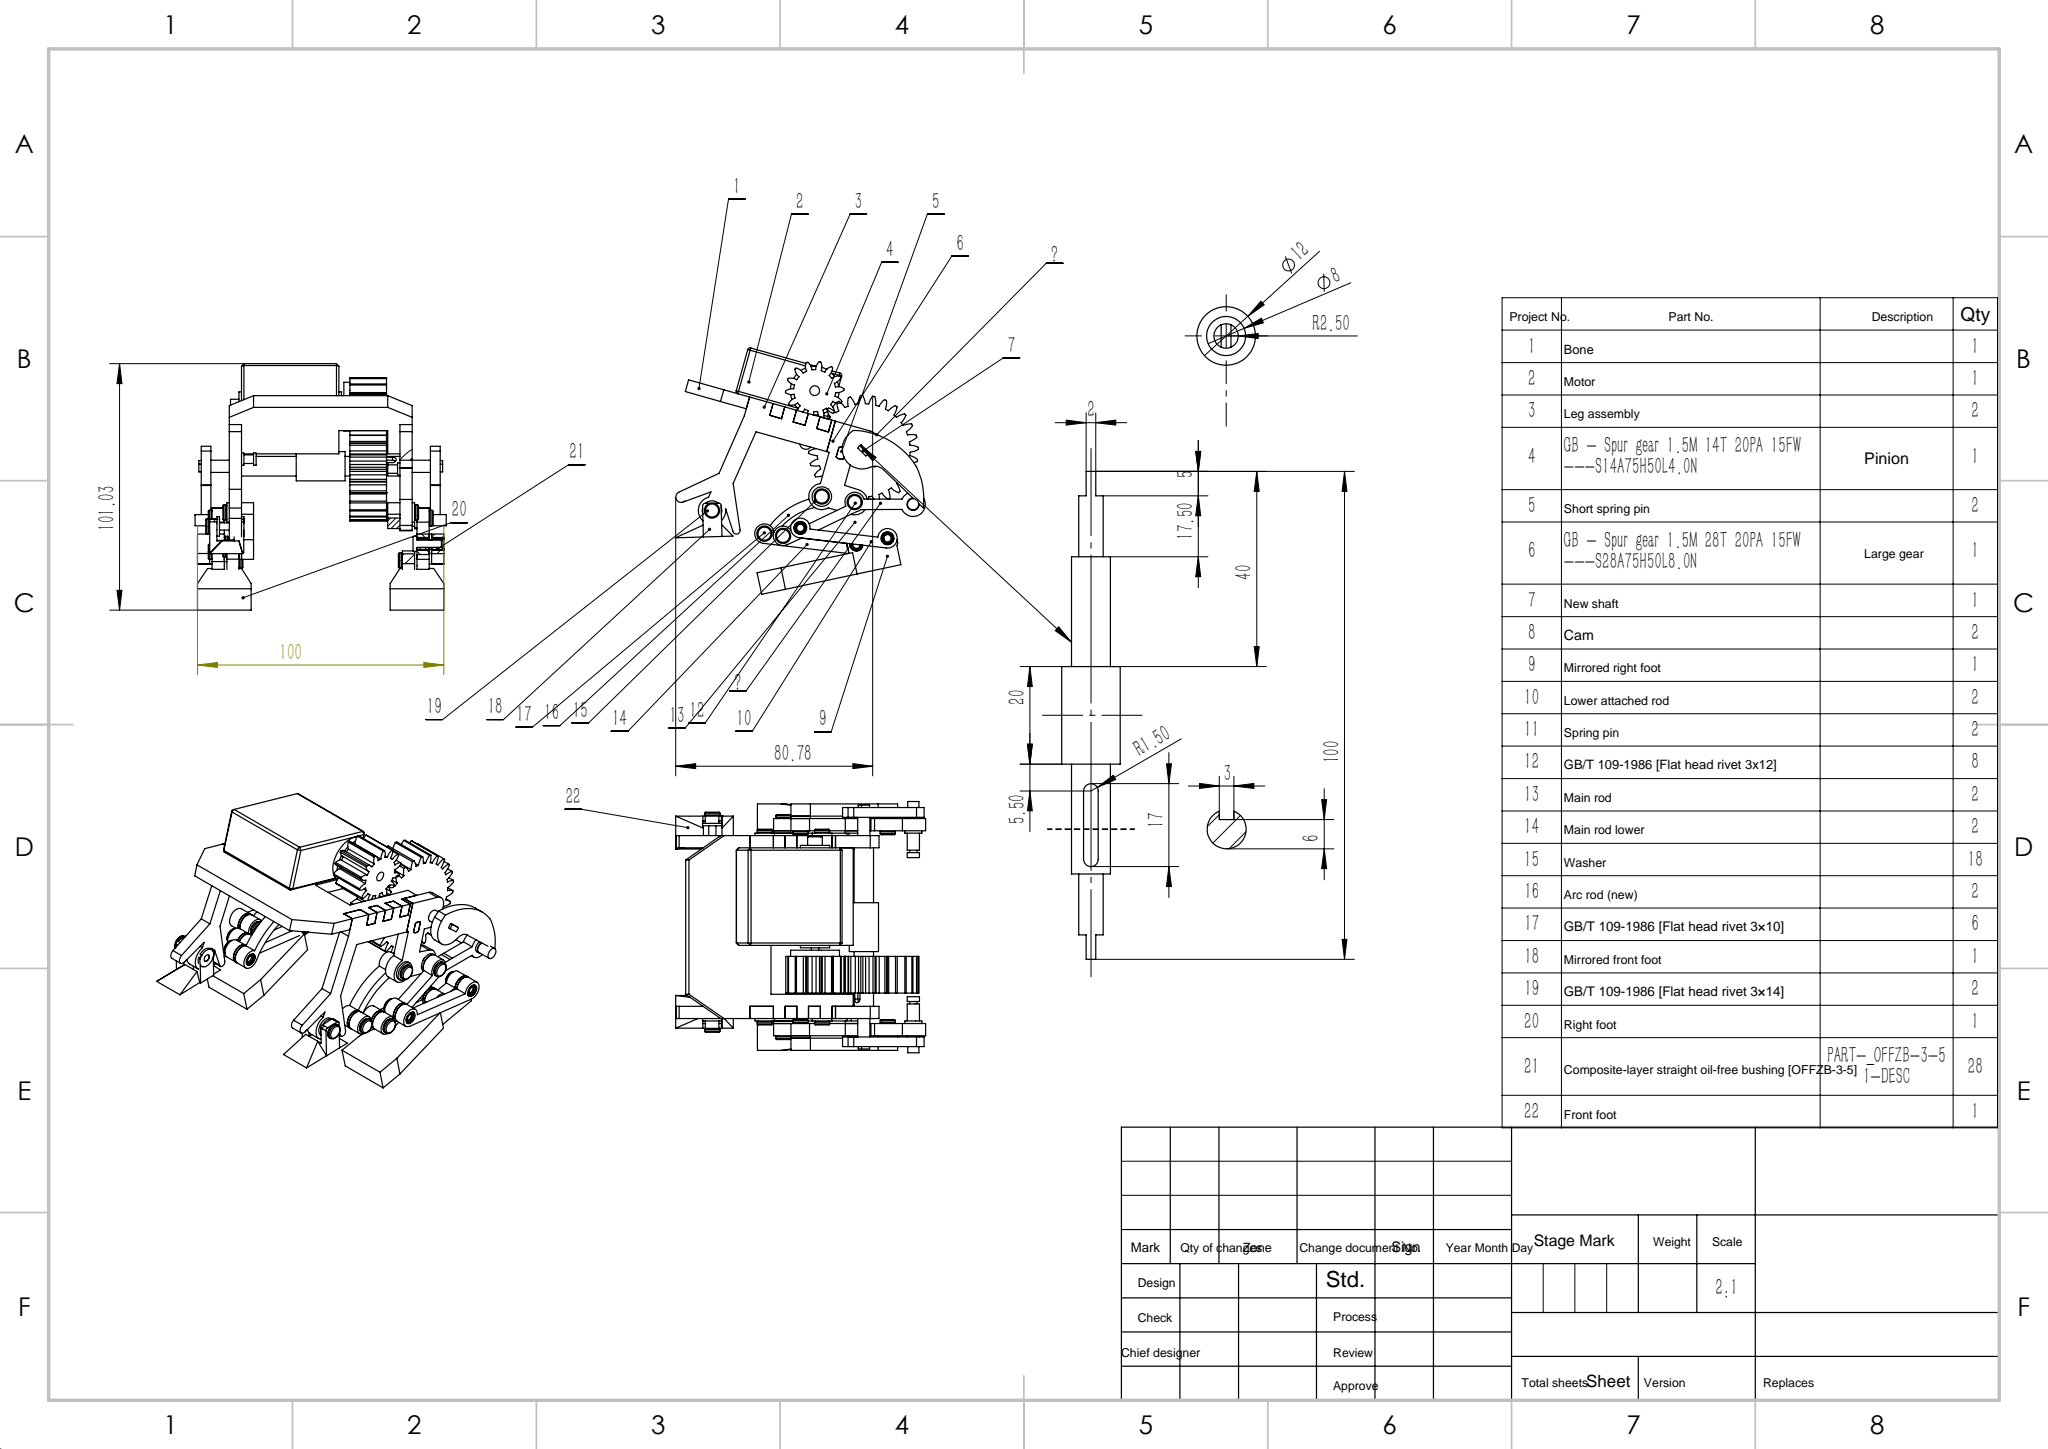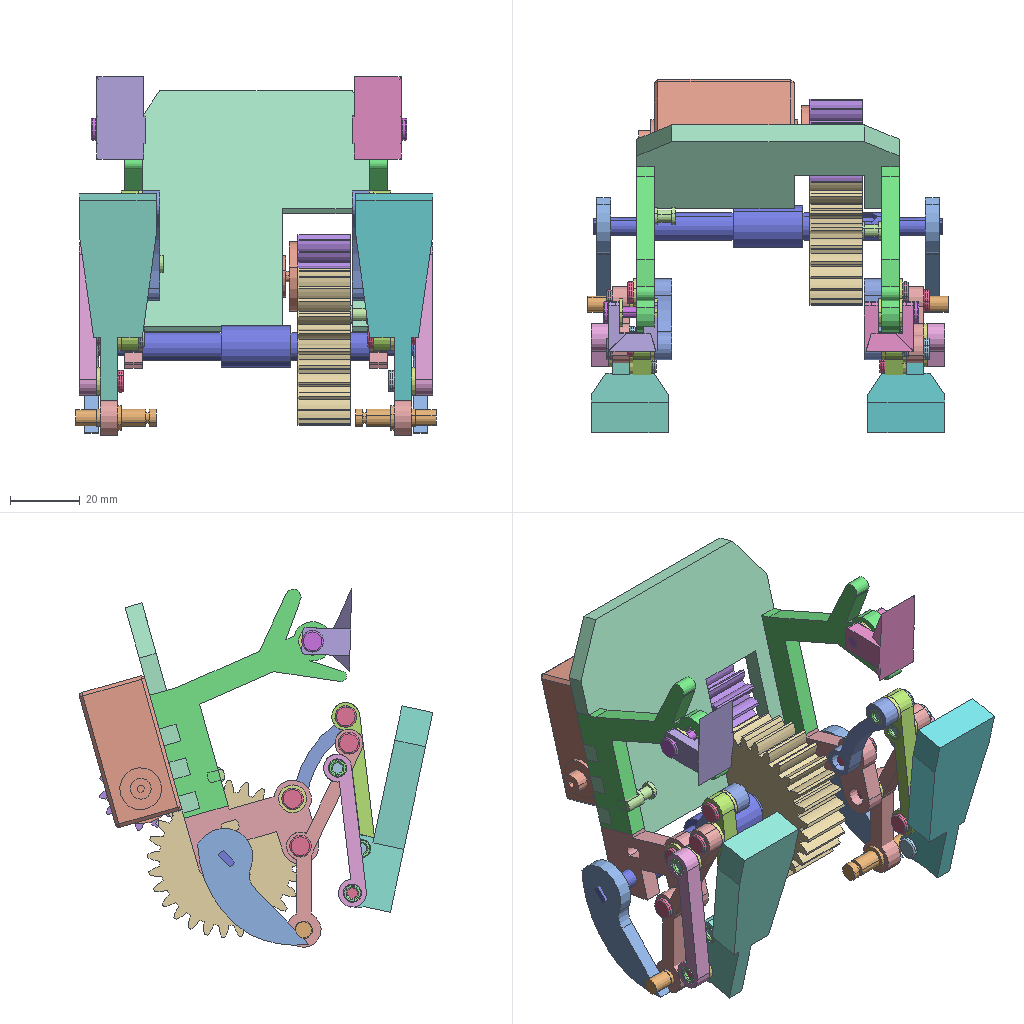Assembly | SolidWorks | 24 different items | 92 placed | box 103 x 101 x 102 mm
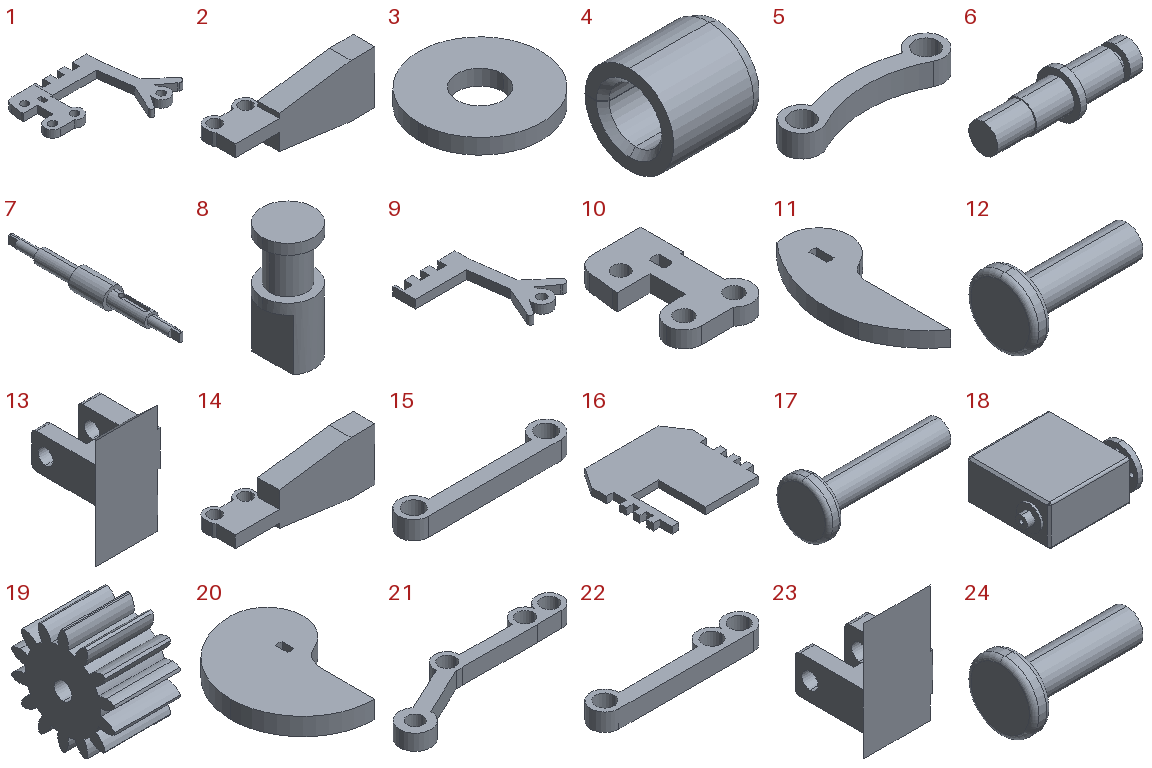Parts list (item | name | quantity | parent item | size | volume | features):
1 | (subassembly) | x2 | - | 76.53 x 55.606 x 5 mm | 6927 mm3 | -
2 | - | x1 | - | 59.063 x 15.813 x 22 mm | 7989 mm3 | features ICE 22, Fillet 4, Attribute 1, Extrusion 1, RevCut 1
3 | - | x18 | - | 8 x 8 x 1 mm | 43.197 mm3 | features Attribute 1, Extrusion 1
4 | - | x28 | - | 5 x 5 x 5 mm | 60.695 mm3 | features MBimport 1
5 | - | x2 | - | 36 x 8 x 5 mm | 695.737 mm3 | features ICE 5, Attribute 1, Extrusion 1
6 | - | x2 | - | 23 x 7 x 7 mm | 439.791 mm3 | features ICE 4, Revolution 2, Attribute 1, Extrusion 1, RevCut 1
7 | - | x1 | - | 12 x 100 x 12 mm | 5018 mm3 | features ICE 7, Extrusion 1
8 | - | x2 | - | 5 x 5 x 11 mm | 147.973 mm3 | features ICE 2, Attribute 1, Extrusion 1
9 | - | x2 | in 1 | 54.608 x 55.606 x 5 mm | 4241 mm3 | features ICE 28, Join 2
10 | - | x2 | in 1 | 24.195 x 36.595 x 5 mm | 2687 mm3 | features ICE 27, Join 2
11 | - | x2 | - | 19.397 x 42.95 x 4 mm | 1803 mm3 | features ICE 4, MirrorStock 1
12 | - | x8 | - | 11.6 x 6.24 x 6.24 mm | 118.025 mm3 | features Revolution 1
13 | - | x1 | - | 14 x 13.739 x 23.602 mm | 1371 mm3 | features MirrorStock 1
14 | - | x1 | - | 59.063 x 15.813 x 22 mm | 7989 mm3 | features MirrorStock 1
15 | - | x2 | - | 44 x 8.023 x 5 mm | 880.516 mm3 | features ICE 10, Fillet 4, Attribute 1, Extrusion 1
16 | - | x1 | - | 75 x 70 x 5 mm | 20550 mm3 | features ICE 5, Attribute 1, Extrusion 1
17 | - | x2 | - | 15.6 x 6.24 x 6.24 mm | 146.299 mm3 | features Revolution 1
18 | - | x1 | - | 49 x 41 x 20 mm | 32126 mm3 | features ICE 7, Chamfer 1, Extrusion 1, Fillet 1
19 | - | x2 | - | 15 x 23.532 x 24 mm | 4730 mm3 | features Boss 3, Cut 3, CirPattern 2, Fillet 2, Revolution 1
20 | - | x1 | - | 24.525 x 32.7 x 4 mm | 2093 mm3 | features ICE 4, Attribute 1, Extrusion 1, Fillet 1
21 | - | x2 | - | 62.758 x 20.04 x 5 mm | 1442 mm3 | features ICE 19, Attribute 1, Extrusion 1
22 | - | x2 | - | 46 x 8 x 5 mm | 936.72 mm3 | features ICE 13, RevCut 2, Attribute 1, Extrusion 1
23 | - | x1 | - | 14 x 13.739 x 23.602 mm | 1371 mm3 | features ICE 19, Fillet 10, Attribute 1, Extrusion 1
24 | - | x6 | - | 11.6 x 6.24 x 6.24 mm | 118.025 mm3 | features Revolution 1
Mates (type | each side: item.copy, entity, surface, feature):
Concentric | 21.1 face cylinder Cut-Extrude6 | 15.1 face cylinder Cut-Extrude4
Concentric | 21.1 face cylinder Cut-Extrude5 | 22.1 face cylinder Cut-Extrude3
Concentric | 5.1 face cylinder Cut-Extrude2 | 22.1 face cylinder Cut-Extrude2
Coincident | 2.1 face plane Boss-Extrude1 | 4.1 face plane Composite-layer straight-column oil-free bushing [OFFZB-3-5].step<1> | 2 times
Concentric | 22.1 face cylinder Cut-Extrude4 | 4.2 face cylinder Composite-layer straight-column oil-free bushing [OFFZB-3-5].step<1>
Coincident | 22.1 face plane Boss-Extrude1 | 4.2 face plane Composite-layer straight-column oil-free bushing [OFFZB-3-5].step<1>
Concentric | 22.1 face cylinder Cut-Extrude3 | 4.3 face cylinder Composite-layer straight-column oil-free bushing [OFFZB-3-5].step<1>
Coincident | 22.1 face plane Boss-Extrude1 | 4.3 face plane Composite-layer straight-column oil-free bushing [OFFZB-3-5].step<1>
Concentric | 5.1 face cylinder Cut-Extrude2 | 4.4 face cylinder Composite-layer straight-column oil-free bushing [OFFZB-3-5].step<1>
Coincident | 5.1 face plane Boss-Extrude1 | 4.4 face plane Composite-layer straight-column oil-free bushing [OFFZB-3-5].step<1>
Concentric | 5.1 face cylinder Cut-Extrude2 | 4.5 face cylinder Composite-layer straight-column oil-free bushing [OFFZB-3-5].step<1>
Coincident | 5.1 face plane Boss-Extrude1 | 4.5 face plane Composite-layer straight-column oil-free bushing [OFFZB-3-5].step<1>
Concentric | 15.1 face cylinder Cut-Extrude3 | 4.6 face cylinder Composite-layer straight-column oil-free bushing [OFFZB-3-5].step<1>
Coincident | 15.1 face plane Boss-Extrude3 | 4.6 face plane Composite-layer straight-column oil-free bushing [OFFZB-3-5].step<1>
Coincident | 2.1 face plane Cut-Extrude3 | 4.7 face plane Composite-layer straight-column oil-free bushing [OFFZB-3-5].step<1>
Concentric | 21.1 face cylinder Cut-Extrude5 | 4.8 face cylinder Composite-layer straight-column oil-free bushing [OFFZB-3-5].step<1>
Coincident | 21.1 face plane Boss-Extrude1 | 4.8 face plane Composite-layer straight-column oil-free bushing [OFFZB-3-5].step<1>
Concentric | 22.1 face cylinder Cut-Extrude2 | 4.9 face cylinder Composite-layer straight-column oil-free bushing [OFFZB-3-5].step<1>
Coincident | 22.1 face plane Boss-Extrude1 | 4.9 face plane Composite-layer straight-column oil-free bushing [OFFZB-3-5].step<1>
Concentric | 21.1 face cylinder Cut-Extrude5 | 4.10 face cylinder Composite-layer straight-column oil-free bushing [OFFZB-3-5].step<1>
Coincident | 21.1 face plane Boss-Extrude1 | 4.10 face plane Composite-layer straight-column oil-free bushing [OFFZB-3-5].step<1>
Concentric | 4.6 face cylinder Composite-layer straight-column oil-free bushing [OFFZB-3-5].step<1> | 12.1 face cylinder Revolve3
Concentric | 4.10 face cylinder Composite-layer straight-column oil-free bushing [OFFZB-3-5].step<1> | 12.2 face cylinder Revolve3
Coincident | 21.1 face plane Boss-Extrude1 | 12.2 face plane Revolve3
Concentric | 4.8 face cylinder Composite-layer straight-column oil-free bushing [OFFZB-3-5].step<1> | 12.3 face cylinder Revolve3
Coincident | 21.1 face plane Boss-Extrude1 | 12.3 face plane Revolve3
Concentric | 4.9 face cylinder Composite-layer straight-column oil-free bushing [OFFZB-3-5].step<1> | 12.4 face cylinder Revolve3
Coincident | 22.1 face plane Boss-Extrude1 | 12.4 face plane Revolve3
Concentric | 4.11 face cylinder Composite-layer straight-column oil-free bushing [OFFZB-3-5].step<1> | 12.5 face cylinder Revolve3
Concentric | 4.2 face cylinder Composite-layer straight-column oil-free bushing [OFFZB-3-5].step<1> | 24.1 face cylinder Revolve3
Coincident | 22.1 face plane Boss-Extrude1 | 24.1 edge
Concentric | 21.1 face cylinder Cut-Extrude6 | 4.12 face cylinder Composite-layer straight-column oil-free bushing [OFFZB-3-5].step<1>
Coincident | 21.1 face plane Boss-Extrude1 | 4.12 face plane Composite-layer straight-column oil-free bushing [OFFZB-3-5].step<1>
Concentric | 15.1 face cylinder Cut-Extrude4 | 4.13 face cylinder Composite-layer straight-column oil-free bushing [OFFZB-3-5].step<1>
Coincident | 15.1 face plane Boss-Extrude3 | 4.13 face plane Composite-layer straight-column oil-free bushing [OFFZB-3-5].step<1>
Concentric | 4.13 face cylinder Composite-layer straight-column oil-free bushing [OFFZB-3-5].step<1> | 24.2 face cylinder Revolve3
Concentric | 4.14 face cylinder Composite-layer straight-column oil-free bushing [OFFZB-3-5].step<1> | 12.2 face cylinder Revolve3
Concentric | 5.1 face cylinder Cut-Extrude2 | 12.5 face cylinder Revolve3
Concentric | 2.1 face cylinder Cut-Extrude12 | 12.1 face cylinder Revolve3
Concentric | 2.1 face cylinder Cut-Extrude12 | 4.1 face cylinder Composite-layer straight-column oil-free bushing [OFFZB-3-5].step<1>
Concentric | 2.1 face cylinder Cut-Extrude12 | 4.7 face cylinder Composite-layer straight-column oil-free bushing [OFFZB-3-5].step<1>
Coincident | 2.1 face plane Boss-Extrude1 | 4.7 face plane Composite-layer straight-column oil-free bushing [OFFZB-3-5].step<1>
Concentric | 4.7 face cylinder Composite-layer straight-column oil-free bushing [OFFZB-3-5].step<1> | 24.1 face cylinder Revolve3
Coincident | 23.1 face plane Cut-Extrude15 | 3.1 face plane Boss-Extrude1
Concentric | 12.5 face cylinder Revolve3 | 3.2 face cylinder Boss-Extrude1
Coincident | 5.1 face plane Boss-Extrude1 | 3.3 face plane Boss-Extrude1
Concentric | 12.4 face cylinder Revolve3 | 3.3 face cylinder Boss-Extrude1
Coincident | 22.1 face plane Boss-Extrude1 | 3.3 face plane Boss-Extrude1
Concentric | 12.2 face cylinder Revolve3 | 3.4 face cylinder Boss-Extrude1
Coincident | 21.1 face plane Boss-Extrude1 | 3.4 face plane Boss-Extrude1
Coincident | 22.1 face plane Boss-Extrude1 | 3.5 face plane Boss-Extrude1
Concentric | 12.3 face cylinder Revolve3 | 3.5 face cylinder Boss-Extrude1
Coincident | 21.1 face plane Boss-Extrude1 | 3.6 face plane Boss-Extrude1
Concentric | 24.2 face cylinder Revolve3 | 3.6 face cylinder Boss-Extrude1
Coincident | 15.1 face plane Boss-Extrude3 | 3.6 face plane Boss-Extrude1
Coincident | 2.1 face plane Cut-Extrude3 | 3.7 face plane Boss-Extrude1
Concentric | 12.1 face cylinder Revolve3 | 3.7 face cylinder Boss-Extrude1
Coincident | 15.1 face plane Boss-Extrude3 | 3.7 face plane Boss-Extrude1
Coincident | 22.1 face plane Boss-Extrude1 | 3.8 face plane Boss-Extrude1
Concentric | 24.1 face cylinder Revolve3 | 3.8 face cylinder Boss-Extrude1
Concentric | 23.1 face cylinder Cut-Extrude1 | 17.1 face cylinder Revolve3
Coincident | 23.1 face plane Boss-Extrude6 | 17.1 face plane Revolve3
Concentric | 4.15 face cylinder Composite-layer straight-column oil-free bushing [OFFZB-3-5].step<1> | 3.9 face cylinder Boss-Extrude1
Concentric | 4.15 face cylinder Composite-layer straight-column oil-free bushing [OFFZB-3-5].step<1> | 17.1 face cylinder Revolve3
Coincident | 16.1 face plane Boss-Extrude1 | 18.1 face plane Boss-Extrude1
DistanceDim | 18.1 face plane Boss-Extrude1 | 16.1 face plane Boss-Extrude1
Concentric | 3.1 face cylinder Boss-Extrude1 | 17.1 face cylinder Revolve3
Concentric | 17.2 face cylinder Revolve3 | 3.10 face cylinder Boss-Extrude1
Concentric | 17.2 face cylinder Revolve3 | 3.11 face cylinder Boss-Extrude1
Concentric | 17.2 face cylinder Revolve3 | 13.1 face cylinder Front Foot_Mirror
Coincident | 3.10 face plane Boss-Extrude1 | 13.1 face plane Front Foot_Mirror
Concentric | 12.6 face cylinder Revolve3 | 4.16 face cylinder Composite-layer straight-column oil-free bushing [OFFZB-3-5].step<1>
Concentric | 12.6 face cylinder Revolve3 | 3.12 face cylinder Boss-Extrude1
Concentric | 12.6 face cylinder Revolve3 | 5.2 face cylinder Cut-Extrude2
Concentric | 12.6 face cylinder Revolve3 | 4.17 face cylinder Composite-layer straight-column oil-free bushing [OFFZB-3-5].step<1>
Concentric | 21.2 face cylinder Cut-Extrude5 | 4.18 face cylinder Composite-layer straight-column oil-free bushing [OFFZB-3-5].step<1>
Coincident | 21.2 face plane Boss-Extrude1 | 4.18 face plane Composite-layer straight-column oil-free bushing [OFFZB-3-5].step<1>
Concentric | 12.7 face cylinder Revolve3 | 3.13 face cylinder Boss-Extrude1
Coincident | 21.2 face plane Boss-Extrude1 | 3.13 face plane Boss-Extrude1
Coincident | 12.7 edge | 21.2 face plane Boss-Extrude1
Coincident | 15.2 face plane Boss-Extrude3 | 3.14 face plane Boss-Extrude1
Coincident | 15.2 face plane Boss-Extrude3 | 4.19 face plane Composite-layer straight-column oil-free bushing [OFFZB-3-5].step<1>
Concentric | 21.2 face cylinder Cut-Extrude6 | 4.20 face cylinder Composite-layer straight-column oil-free bushing [OFFZB-3-5].step<1>
Coincident | 21.2 face plane Boss-Extrude1 | 4.20 face plane Composite-layer straight-column oil-free bushing [OFFZB-3-5].step<1>
Coincident | 21.2 face plane Boss-Extrude1 | 3.14 face plane Boss-Extrude1
Coincident | 5.2 face plane Boss-Extrude1 | 4.21 face plane Composite-layer straight-column oil-free bushing [OFFZB-3-5].step<1>
Concentric | 5.2 face cylinder Cut-Extrude2 | 4.21 face cone Composite-layer straight-column oil-free bushing [OFFZB-3-5].step<1>
Coincident | 4.22 face plane Composite-layer straight-column oil-free bushing [OFFZB-3-5].step<1> | 22.2 face plane Boss-Extrude1
Concentric | 4.22 face cylinder Composite-layer straight-column oil-free bushing [OFFZB-3-5].step<1> | 22.2 face cylinder Cut-Extrude2
Concentric | 4.22 face cylinder Composite-layer straight-column oil-free bushing [OFFZB-3-5].step<1> | 24.3 face cylinder Revolve3
Coincident | 22.2 face plane Boss-Extrude1 | 24.3 face plane Revolve3
Coincident | 22.2 face plane Boss-Extrude1 | 3.15 face plane Boss-Extrude1
Concentric | 24.3 face cylinder Revolve3 | 3.15 face cylinder Boss-Extrude1
Concentric | 4.21 face cylinder Composite-layer straight-column oil-free bushing [OFFZB-3-5].step<1> | 24.3 face cylinder Revolve3
Coincident | 5.2 face plane Boss-Extrude1 | 3.15 edge
Coincident | 4.23 face plane Composite-layer straight-column oil-free bushing [OFFZB-3-5].step<1> | 22.2 face plane Boss-Extrude1
Concentric | 4.23 face cylinder Composite-layer straight-column oil-free bushing [OFFZB-3-5].step<1> | 22.2 face cylinder Cut-Extrude3
Coincident | 3.16 face plane Boss-Extrude1 | 22.2 face plane Boss-Extrude1
Concentric | 21.2 face cylinder Cut-Extrude5 | 4.24 face cylinder Composite-layer straight-column oil-free bushing [OFFZB-3-5].step<1>
Coincident | 21.2 face plane Boss-Extrude1 | 4.24 face plane Composite-layer straight-column oil-free bushing [OFFZB-3-5].step<1>
Coincident | 15.2 face plane Boss-Extrude3 | 4.25 face plane Composite-layer straight-column oil-free bushing [OFFZB-3-5].step<1>
Coincident | 15.2 face plane Boss-Extrude3 | 3.17 face plane Boss-Extrude1
Concentric | 22.2 face cylinder Cut-Extrude4 | 4.26 face cylinder Composite-layer straight-column oil-free bushing [OFFZB-3-5].step<1>
Coincident | 22.2 face plane Boss-Extrude1 | 4.26 face plane Composite-layer straight-column oil-free bushing [OFFZB-3-5].step<1>
Concentric | 4.26 face cylinder Composite-layer straight-column oil-free bushing [OFFZB-3-5].step<1> | 14.1 face cylinder RightFoot_Mirror
Concentric | 14.1 face cylinder RightFoot_Mirror | 4.27 face cylinder Composite-layer straight-column oil-free bushing [OFFZB-3-5].step<1>
Coincident | 14.1 face plane RightFoot_Mirror | 4.27 face plane Composite-layer straight-column oil-free bushing [OFFZB-3-5].step<1>
Concentric | 14.1 face cylinder RightFoot_Mirror | 4.28 face cylinder Composite-layer straight-column oil-free bushing [OFFZB-3-5].step<1>
Coincident | 14.1 face plane RightFoot_Mirror | 4.28 face plane Composite-layer straight-column oil-free bushing [OFFZB-3-5].step<1>
Concentric | 4.26 face cylinder Composite-layer straight-column oil-free bushing [OFFZB-3-5].step<1> | 12.8 face cylinder Revolve3
Coincident | 22.2 face plane Boss-Extrude1 | 12.8 face plane Revolve3
Concentric | 12.8 face cylinder Revolve3 | 3.18 face cylinder Boss-Extrude1
Coincident | 22.2 face plane Boss-Extrude1 | 3.18 face plane Boss-Extrude1
Coincident | 3.17 face plane Boss-Extrude1 | 14.1 face plane RightFoot_Mirror
Concentric | 4.24 face cylinder Composite-layer straight-column oil-free bushing [OFFZB-3-5].step<1> | 24.4 face cylinder Revolve3
Concentric | 3.16 face cylinder Boss-Extrude1 | 24.4 face cylinder Revolve3
Concentric | 4.23 face cylinder Composite-layer straight-column oil-free bushing [OFFZB-3-5].step<1> | 24.4 face cylinder Revolve3
Coincident | 21.2 face plane Boss-Extrude1 | 24.4 face plane Revolve3
Parallel | 18.1 face plane Boss-Extrude6 | 19.1 face plane Base-Revolve
Coincident | 18.1 face plane Boss-Extrude6 | 19.1 face plane Base-Revolve
Concentric | 7.1 face cylinder Boss-Extrude4 | 19.2 face cylinder Bore
Coincident | 19.2 face plane Base-Revolve | 19.1 face plane Base-Revolve
GearDim | 19.1 face cylinder TeethCuts | 19.2 face cylinder TeethCuts
Concentric | 18.1 edge | 19.1 edge
Parallel | 2.1 face plane Boss-Extrude12 | 14.1 face plane RightFoot_Mirror
Coincident | 16.1 face plane Cut-Extrude3 | 9.1 face plane Cut-Extrude12
Coincident | 16.1 face plane Boss-Extrude1 | 9.1 face plane Join 1 | 2 times
Coincident | 17.2 face plane Revolve3 | 13.1 face plane Front Foot_Mirror
Concentric | 17.2 face cylinder Revolve3 | 9.1 face cylinder Join 2
Coincident | 3.10 face plane Boss-Extrude1 | 9.1 face plane Join 1
Concentric | 12.6 face cylinder Revolve3 | 10.1 face cylinder Cut-Extrude7
Concentric | 4.18 face cylinder Composite-layer straight-column oil-free bushing [OFFZB-3-5].step<1> | 10.1 edge
Coincident | 8.1 face plane Cut-Extrude1 | 10.1 face plane Cut-Extrude11
Concentric | 8.1 face cylinder Boss-Extrude1 | 10.1 face cylinder Cut-Extrude11
Coincident | 8.1 face plane Boss-Extrude1 | 10.1 face plane Join 1
Concentric | 7.1 face cylinder Boss-Extrude5 | 10.1 face cylinder Join 1
Concentric | 12.7 face cylinder Revolve3 | 4.18 face cylinder Composite-layer straight-column oil-free bushing [OFFZB-3-5].step<1>
Coincident | 7.1 face plane Boss-Extrude4 | 10.1 edge
Coincident | 21.2 face plane Boss-Extrude1 | 3.16 face plane Boss-Extrude1
Coincident | 16.1 face plane Boss-Extrude1 | 10.2 face plane Join 1
Coincident | 16.1 face plane Boss-Extrude1 | 9.2 edge
Coincident | 16.1 face plane Cut-Extrude4 | 9.2 face plane Cut-Extrude12
Concentric | 17.1 face cylinder Revolve3 | 9.2 face cylinder Join 2
Concentric | 12.5 face cylinder Revolve3 | 10.2 face cylinder Cut-Extrude7
Coincident | 21.1 edge | 3.5 face plane Boss-Extrude1
Coincident | 4.14 face plane Composite-layer straight-column oil-free bushing [OFFZB-3-5].step<1> | 3.4 face plane Boss-Extrude1
Concentric | 4.14 face cylinder Composite-layer straight-column oil-free bushing [OFFZB-3-5].step<1> | 10.2 face cylinder Join 1
Coincident | 5.2 face plane Boss-Extrude1 | 10.1 face plane Join 1
Coincident | 3.12 face plane Boss-Extrude1 | 10.1 face plane Join 1
Coincident | 3.12 face plane Boss-Extrude1 | 4.17 edge
Coincident | 12.6 face plane Revolve3 | 3.12 face plane Boss-Extrude1
Coincident | 5.1 face plane Boss-Extrude1 | 10.2 face plane Join 1
Coincident | 3.2 face plane Boss-Extrude1 | 10.2 face plane Join 1
Coincident | 12.5 face plane Revolve3 | 3.2 face plane Boss-Extrude1
DistanceDim | 16.1 face plane Cut-Extrude5 | 18.1 face plane Boss-Extrude1
Coincident | 23.1 face plane Cut-Extrude17 | 13.1 face plane Front Foot_Mirror
Concentric | 24.5 face cylinder Revolve3 | 4.27 face cylinder Composite-layer straight-column oil-free bushing [OFFZB-3-5].step<1>
Coincident | 24.5 face plane Revolve3 | 14.1 face plane RightFoot_Mirror
Concentric | 15.2 face cylinder Cut-Extrude3 | 4.25 face cylinder Composite-layer straight-column oil-free bushing [OFFZB-3-5].step<1>
Coincident | 24.5 face cylinder Revolve3 | 4.25 edge
Concentric | 24.6 face cylinder Revolve3 | 4.19 edge
Coincident | 21.2 face plane Boss-Extrude1 | 24.6 face plane Revolve3
Concentric | 15.2 edge | 4.19 face cylinder Composite-layer straight-column oil-free bushing [OFFZB-3-5].step<1>
Coincident | 4.20 face cylinder Composite-layer straight-column oil-free bushing [OFFZB-3-5].step<1> | 4.19 edge
Tangent | 3.17 face cylinder Boss-Extrude1 | 24.5 face cylinder Revolve3
Coincident | 24.6 face cylinder Revolve3 | 3.14 edge
Coincident | 21.1 face plane Boss-Extrude1 | 24.2 face plane Revolve3
Coincident | 2.1 face plane Boss-Extrude1 | 12.1 face plane Revolve3
Coincident | 21.2 face plane Boss-Extrude1 | 6.1 face plane Revolve2
Concentric | 21.2 face cylinder Boss-Extrude16 | 6.1 face cylinder Revolve1
Concentric | 21.1 face cylinder Boss-Extrude16 | 6.2 face cylinder Revolve1
Coincident | 21.1 face plane Boss-Extrude1 | 6.2 face plane Revolve2
Coincident | 7.1 face plane Boss-Extrude6 | 11.1 face plane Cut-Extrude1
Coincident | 11.1 face plane tu_Mirror | 7.1 face plane Boss-Extrude5
Concentric | 7.1 face cylinder Boss-Extrude5 | 11.1 face cylinder Cut-Extrude1
Concentric | 7.1 face cylinder Boss-Extrude3 | 11.2 face cylinder Cut-Extrude1
Coincident | 7.1 face plane Boss-Extrude7 | 11.2 face plane Cut-Extrude1
Coincident | 7.1 face plane Boss-Extrude3 | 11.2 face plane tu_Mirror